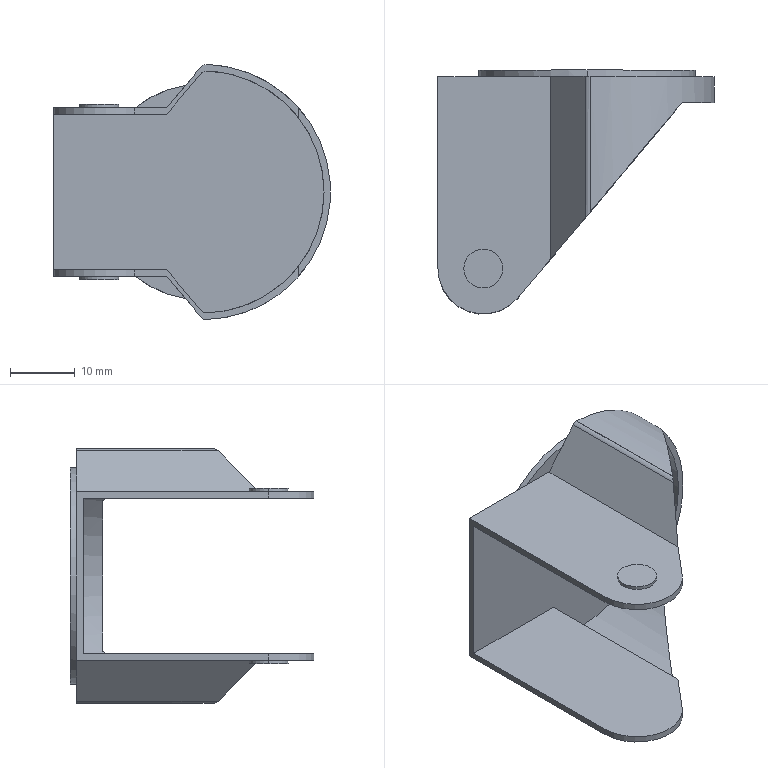Part | STEP file | CLGJ50_Rbody | 1 solid | 36 faces | box 42.667 x 37.625 x 39.322 mm | volume 4018 mm3 | plane 20 | cylinder 16 | commonest cylinder face diameters 2 x6 6 x4 14 x2 33.333 x2 37.333 x1 39.333 x1
STEP:
#1=CARTESIAN_POINT('',(-13.,-40.,-13.5));
#2=VERTEX_POINT('',#1);
#3=CARTESIAN_POINT('',(-19.,-40.,-13.5));
#4=VERTEX_POINT('',#3);
#5=CARTESIAN_POINT('',(-16.,-40.,-13.5));
#6=DIRECTION('',(0.,0.,1.));
#7=DIRECTION('',(1.,0.,0.));
#8=AXIS2_PLACEMENT_3D('',#5,#6,#7);
#9=CIRCLE('',#8,3.);
#10=EDGE_CURVE('',#2,#4,#9,.T.);
#11=ORIENTED_EDGE('',*,*,#10,.T.);
#12=CARTESIAN_POINT('',(-19.,-40.,-13.));
#13=VERTEX_POINT('',#12);
#14=CARTESIAN_POINT('',(-19.,-40.,-13.5));
#15=DIRECTION('',(0.,0.,1.));
#16=VECTOR('',#15,1000.);
#17=LINE('',#14,#16);
#18=EDGE_CURVE('',#4,#13,#17,.T.);
#19=ORIENTED_EDGE('',*,*,#18,.T.);
#20=CARTESIAN_POINT('',(-13.,-40.,-13.));
#21=VERTEX_POINT('',#20);
#22=CARTESIAN_POINT('',(-16.,-40.,-13.));
#23=DIRECTION('',(0.,0.,-1.));
#24=DIRECTION('',(-1.,0.,0.));
#25=AXIS2_PLACEMENT_3D('',#22,#23,#24);
#26=CIRCLE('',#25,3.);
#27=EDGE_CURVE('',#13,#21,#26,.T.);
#28=ORIENTED_EDGE('',*,*,#27,.T.);
#29=CARTESIAN_POINT('',(-13.,-40.,-13.5));
#30=DIRECTION('',(0.,0.,1.));
#31=VECTOR('',#30,1000.);
#32=LINE('',#29,#31);
#33=EDGE_CURVE('',#2,#21,#32,.T.);
#34=ORIENTED_EDGE('',*,*,#33,.F.);
#35=EDGE_LOOP('',(#11,#19,#28,#34));
#36=FACE_OUTER_BOUND('',#35,.T.);
#37=CARTESIAN_POINT('',(-16.,-40.,-13.5));
#38=DIRECTION('',(0.,0.,1.));
#39=DIRECTION('',(1.,0.,0.));
#40=AXIS2_PLACEMENT_3D('',#37,#38,#39);
#41=CYLINDRICAL_SURFACE('',#40,3.);
#42=ADVANCED_FACE('',(#36),#41,.T.);
#43=CARTESIAN_POINT('',(-13.,-40.,13.5));
#44=VERTEX_POINT('',#43);
#45=CARTESIAN_POINT('',(-19.,-40.,13.5));
#46=VERTEX_POINT('',#45);
#47=CARTESIAN_POINT('',(-16.,-40.,13.5));
#48=DIRECTION('',(0.,0.,1.));
#49=DIRECTION('',(1.,0.,0.));
#50=AXIS2_PLACEMENT_3D('',#47,#48,#49);
#51=CIRCLE('',#50,3.);
#52=EDGE_CURVE('',#44,#46,#51,.T.);
#53=ORIENTED_EDGE('',*,*,#52,.F.);
#54=CARTESIAN_POINT('',(-13.,-40.,13.));
#55=VERTEX_POINT('',#54);
#56=CARTESIAN_POINT('',(-13.,-40.,13.5));
#57=DIRECTION('',(0.,0.,-1.));
#58=VECTOR('',#57,1000.);
#59=LINE('',#56,#58);
#60=EDGE_CURVE('',#44,#55,#59,.T.);
#61=ORIENTED_EDGE('',*,*,#60,.T.);
#62=CARTESIAN_POINT('',(-19.,-40.,13.));
#63=VERTEX_POINT('',#62);
#64=CARTESIAN_POINT('',(-16.,-40.,13.));
#65=DIRECTION('',(0.,0.,1.));
#66=DIRECTION('',(1.,0.,0.));
#67=AXIS2_PLACEMENT_3D('',#64,#65,#66);
#68=CIRCLE('',#67,3.);
#69=EDGE_CURVE('',#55,#63,#68,.T.);
#70=ORIENTED_EDGE('',*,*,#69,.T.);
#71=CARTESIAN_POINT('',(-19.,-40.,13.5));
#72=DIRECTION('',(0.,0.,-1.));
#73=VECTOR('',#72,1000.);
#74=LINE('',#71,#73);
#75=EDGE_CURVE('',#46,#63,#74,.T.);
#76=ORIENTED_EDGE('',*,*,#75,.F.);
#77=EDGE_LOOP('',(#53,#61,#70,#76));
#78=FACE_OUTER_BOUND('',#77,.T.);
#79=CARTESIAN_POINT('',(-16.,-40.,13.5));
#80=DIRECTION('',(0.,0.,-1.));
#81=DIRECTION('',(-1.,0.,0.));
#82=AXIS2_PLACEMENT_3D('',#79,#80,#81);
#83=CYLINDRICAL_SURFACE('',#82,3.);
#84=ADVANCED_FACE('',(#78),#83,.T.);
#85=CARTESIAN_POINT('',(0.4874,-31.255,18.66));
#86=VERTEX_POINT('',#85);
#87=CARTESIAN_POINT('',(0.4613,-31.286,18.661));
#88=VERTEX_POINT('',#87);
#89=CARTESIAN_POINT('',(0.4874,-31.255,18.66));
#90=CARTESIAN_POINT('',(0.4787,-31.266,18.661));
#91=CARTESIAN_POINT('',(0.47,-31.276,18.661));
#92=CARTESIAN_POINT('',(0.4613,-31.286,18.661));
#93=(BOUNDED_CURVE()B_SPLINE_CURVE(3,(#89,#90,#91,#92),.UNSPECIFIED.,.F.,.F.)B_SPLINE_CURVE_WITH_KNOTS((4,4),(1.545,1.571),.UNSPECIFIED.)CURVE()GEOMETRIC_REPRESENTATION_ITEM()RATIONAL_B_SPLINE_CURVE((1.,0.9999,0.9999,1.))REPRESENTATION_ITEM(''));
#94=EDGE_CURVE('',#86,#88,#93,.T.);
#95=ORIENTED_EDGE('',*,*,#94,.T.);
#96=CARTESIAN_POINT('',(0.4613,-11.375,18.661));
#97=VERTEX_POINT('',#96);
#98=CARTESIAN_POINT('',(0.4613,-76.375,18.661));
#99=DIRECTION('',(0.,1.,0.));
#100=VECTOR('',#99,1000.);
#101=LINE('',#98,#100);
#102=EDGE_CURVE('',#88,#97,#101,.T.);
#103=ORIENTED_EDGE('',*,*,#102,.T.);
#104=CARTESIAN_POINT('',(0.4874,-11.375,18.66));
#105=VERTEX_POINT('',#104);
#106=CARTESIAN_POINT('',(0.4613,-11.375,17.661));
#107=DIRECTION('',(0.,1.,0.));
#108=DIRECTION('',(0.,0.,1.));
#109=AXIS2_PLACEMENT_3D('',#106,#107,#108);
#110=CIRCLE('',#109,1.);
#111=EDGE_CURVE('',#97,#105,#110,.T.);
#112=ORIENTED_EDGE('',*,*,#111,.T.);
#113=CARTESIAN_POINT('',(0.4874,-76.375,18.66));
#114=DIRECTION('',(0.,1.,0.));
#115=VECTOR('',#114,1000.);
#116=LINE('',#113,#115);
#117=EDGE_CURVE('',#86,#105,#116,.T.);
#118=ORIENTED_EDGE('',*,*,#117,.F.);
#119=EDGE_LOOP('',(#95,#103,#112,#118));
#120=FACE_OUTER_BOUND('',#119,.T.);
#121=CARTESIAN_POINT('',(0.4613,-76.375,17.661));
#122=DIRECTION('',(0.,1.,0.));
#123=DIRECTION('',(0.,0.,1.));
#124=AXIS2_PLACEMENT_3D('',#121,#122,#123);
#125=CYLINDRICAL_SURFACE('',#124,1.);
#126=ADVANCED_FACE('',(#120),#125,.F.);
#127=CARTESIAN_POINT('',(0.4615,-31.286,19.661));
#128=VERTEX_POINT('',#127);
#129=CARTESIAN_POINT('',(-0.3045,-32.198,19.304));
#130=VERTEX_POINT('',#129);
#131=CARTESIAN_POINT('',(0.4615,-31.286,19.661));
#132=CARTESIAN_POINT('',(0.161,-31.644,19.661));
#133=CARTESIAN_POINT('',(-0.1114,-31.968,19.534));
#134=CARTESIAN_POINT('',(-0.3045,-32.198,19.304));
#135=(BOUNDED_CURVE()B_SPLINE_CURVE(3,(#131,#132,#133,#134),.UNSPECIFIED.,.F.,.F.)B_SPLINE_CURVE_WITH_KNOTS((4,4),(1.571,2.443),.UNSPECIFIED.)CURVE()GEOMETRIC_REPRESENTATION_ITEM()RATIONAL_B_SPLINE_CURVE((1.,0.9375,0.9375,1.))REPRESENTATION_ITEM(''));
#136=EDGE_CURVE('',#128,#130,#135,.T.);
#137=ORIENTED_EDGE('',*,*,#136,.F.);
#138=CARTESIAN_POINT('',(0.4615,-10.375,19.661));
#139=VERTEX_POINT('',#138);
#140=CARTESIAN_POINT('',(0.4615,-54.375,19.661));
#141=DIRECTION('',(0.,1.,0.));
#142=VECTOR('',#141,1000.);
#143=LINE('',#140,#142);
#144=EDGE_CURVE('',#128,#139,#143,.T.);
#145=ORIENTED_EDGE('',*,*,#144,.T.);
#146=CARTESIAN_POINT('',(-0.3045,-10.375,19.304));
#147=VERTEX_POINT('',#146);
#148=CARTESIAN_POINT('',(0.4615,-10.375,18.661));
#149=DIRECTION('',(0.,1.,0.));
#150=DIRECTION('',(0.,0.,1.));
#151=AXIS2_PLACEMENT_3D('',#148,#149,#150);
#152=CIRCLE('',#151,1.);
#153=EDGE_CURVE('',#147,#139,#152,.T.);
#154=ORIENTED_EDGE('',*,*,#153,.F.);
#155=CARTESIAN_POINT('',(-0.3045,-54.375,19.304));
#156=DIRECTION('',(0.,1.,0.));
#157=VECTOR('',#156,1000.);
#158=LINE('',#155,#157);
#159=EDGE_CURVE('',#130,#147,#158,.T.);
#160=ORIENTED_EDGE('',*,*,#159,.F.);
#161=EDGE_LOOP('',(#137,#145,#154,#160));
#162=FACE_OUTER_BOUND('',#161,.T.);
#163=CARTESIAN_POINT('',(0.4615,-54.375,18.661));
#164=DIRECTION('',(0.,1.,0.));
#165=DIRECTION('',(0.,0.,1.));
#166=AXIS2_PLACEMENT_3D('',#163,#164,#165);
#167=CYLINDRICAL_SURFACE('',#166,1.);
#168=ADVANCED_FACE('',(#162),#167,.T.);
#169=CARTESIAN_POINT('',(0.,-10.375,16.667));
#170=VERTEX_POINT('',#169);
#171=CARTESIAN_POINT('',(0.,-10.375,-16.667));
#172=VERTEX_POINT('',#171);
#173=CARTESIAN_POINT('',(0.,-10.375,0.));
#174=DIRECTION('',(0.,1.,0.));
#175=DIRECTION('',(0.,0.,1.));
#176=AXIS2_PLACEMENT_3D('',#173,#174,#175);
#177=CIRCLE('',#176,16.667);
#178=EDGE_CURVE('',#170,#172,#177,.T.);
#179=ORIENTED_EDGE('',*,*,#178,.T.);
#180=CARTESIAN_POINT('',(0.,-9.375,-16.667));
#181=VERTEX_POINT('',#180);
#182=CARTESIAN_POINT('',(0.,-10.375,-16.667));
#183=DIRECTION('',(0.,1.,0.));
#184=VECTOR('',#183,1000.);
#185=LINE('',#182,#184);
#186=EDGE_CURVE('',#172,#181,#185,.T.);
#187=ORIENTED_EDGE('',*,*,#186,.T.);
#188=CARTESIAN_POINT('',(0.,-9.375,16.667));
#189=VERTEX_POINT('',#188);
#190=CARTESIAN_POINT('',(0.,-9.375,0.));
#191=DIRECTION('',(0.,1.,0.));
#192=DIRECTION('',(0.,0.,1.));
#193=AXIS2_PLACEMENT_3D('',#190,#191,#192);
#194=CIRCLE('',#193,16.667);
#195=EDGE_CURVE('',#189,#181,#194,.T.);
#196=ORIENTED_EDGE('',*,*,#195,.F.);
#197=CARTESIAN_POINT('',(0.,-10.375,16.667));
#198=DIRECTION('',(0.,1.,0.));
#199=VECTOR('',#198,1000.);
#200=LINE('',#197,#199);
#201=EDGE_CURVE('',#170,#189,#200,.T.);
#202=ORIENTED_EDGE('',*,*,#201,.F.);
#203=EDGE_LOOP('',(#179,#187,#196,#202));
#204=FACE_OUTER_BOUND('',#203,.T.);
#205=CARTESIAN_POINT('',(0.,-10.375,0.));
#206=DIRECTION('',(0.,1.,0.));
#207=DIRECTION('',(0.,0.,1.));
#208=AXIS2_PLACEMENT_3D('',#205,#206,#207);
#209=CYLINDRICAL_SURFACE('',#208,16.667);
#210=ADVANCED_FACE('',(#204),#209,.T.);
#211=CARTESIAN_POINT('',(-10.64,-44.502,13.));
#212=VERTEX_POINT('',#211);
#213=CARTESIAN_POINT('',(-23.,-40.,13.));
#214=VERTEX_POINT('',#213);
#215=CARTESIAN_POINT('',(-16.,-40.,13.));
#216=DIRECTION('',(0.,0.,-1.));
#217=DIRECTION('',(1.,0.,0.));
#218=AXIS2_PLACEMENT_3D('',#215,#216,#217);
#219=CIRCLE('',#218,7.);
#220=EDGE_CURVE('',#212,#214,#219,.T.);
#221=ORIENTED_EDGE('',*,*,#220,.F.);
#222=CARTESIAN_POINT('',(-5.594,-38.495,13.));
#223=VERTEX_POINT('',#222);
#224=CARTESIAN_POINT('',(-20.615,-56.378,13.));
#225=DIRECTION('',(-0.6432,-0.7657,0.));
#226=VECTOR('',#225,1000.);
#227=LINE('',#224,#226);
#228=EDGE_CURVE('',#223,#212,#227,.T.);
#229=ORIENTED_EDGE('',*,*,#228,.F.);
#230=CARTESIAN_POINT('',(-5.594,-10.375,13.));
#231=VERTEX_POINT('',#230);
#232=CARTESIAN_POINT('',(-5.594,-54.375,13.));
#233=DIRECTION('',(0.,1.,0.));
#234=VECTOR('',#233,1000.);
#235=LINE('',#232,#234);
#236=EDGE_CURVE('',#223,#231,#235,.T.);
#237=ORIENTED_EDGE('',*,*,#236,.T.);
#238=CARTESIAN_POINT('',(-10.43,-10.375,13.));
#239=VERTEX_POINT('',#238);
#240=CARTESIAN_POINT('',(-23.,-10.375,13.));
#241=DIRECTION('',(1.,0.,0.));
#242=VECTOR('',#241,1000.);
#243=LINE('',#240,#242);
#244=EDGE_CURVE('',#239,#231,#243,.T.);
#245=ORIENTED_EDGE('',*,*,#244,.F.);
#246=CARTESIAN_POINT('',(-23.,-10.375,13.));
#247=VERTEX_POINT('',#246);
#248=CARTESIAN_POINT('',(-23.,-10.375,13.));
#249=DIRECTION('',(1.,0.,0.));
#250=VECTOR('',#249,1000.);
#251=LINE('',#248,#250);
#252=EDGE_CURVE('',#247,#239,#251,.T.);
#253=ORIENTED_EDGE('',*,*,#252,.F.);
#254=CARTESIAN_POINT('',(-23.,-54.375,13.));
#255=DIRECTION('',(0.,1.,0.));
#256=VECTOR('',#255,1000.);
#257=LINE('',#254,#256);
#258=EDGE_CURVE('',#214,#247,#257,.T.);
#259=ORIENTED_EDGE('',*,*,#258,.F.);
#260=EDGE_LOOP('',(#221,#229,#237,#245,#253,#259));
#261=FACE_OUTER_BOUND('',#260,.T.);
#262=CARTESIAN_POINT('',(-16.,-40.,13.));
#263=DIRECTION('',(0.,0.,1.));
#264=DIRECTION('',(1.,0.,0.));
#265=AXIS2_PLACEMENT_3D('',#262,#263,#264);
#266=CIRCLE('',#265,3.);
#267=EDGE_CURVE('',#63,#55,#266,.T.);
#268=ORIENTED_EDGE('',*,*,#267,.F.);
#269=ORIENTED_EDGE('',*,*,#69,.F.);
#270=EDGE_LOOP('',(#268,#269));
#271=FACE_BOUND('',#270,.T.);
#272=CARTESIAN_POINT('',(-23.,-54.375,13.));
#273=DIRECTION('',(0.,0.,1.));
#274=DIRECTION('',(1.,0.,0.));
#275=AXIS2_PLACEMENT_3D('',#272,#273,#274);
#276=PLANE('',#275);
#277=ADVANCED_FACE('',(#261,#271),#276,.T.);
#278=CARTESIAN_POINT('',(-2.702,-10.375,16.446));
#279=VERTEX_POINT('',#278);
#280=CARTESIAN_POINT('',(0.,-10.375,0.));
#281=DIRECTION('',(0.,1.,0.));
#282=DIRECTION('',(0.,0.,1.));
#283=AXIS2_PLACEMENT_3D('',#280,#281,#282);
#284=CIRCLE('',#283,16.667);
#285=EDGE_CURVE('',#239,#279,#284,.T.);
#286=ORIENTED_EDGE('',*,*,#285,.F.);
#287=ORIENTED_EDGE('',*,*,#244,.T.);
#288=CARTESIAN_POINT('',(-5.594,-10.375,13.));
#289=DIRECTION('',(0.6428,0.,0.766));
#290=VECTOR('',#289,1000.);
#291=LINE('',#288,#290);
#292=EDGE_CURVE('',#231,#279,#291,.T.);
#293=ORIENTED_EDGE('',*,*,#292,.T.);
#294=EDGE_LOOP('',(#286,#287,#293));
#295=FACE_OUTER_BOUND('',#294,.T.);
#296=CARTESIAN_POINT('',(0.,-10.375,0.));
#297=DIRECTION('',(0.,1.,0.));
#298=DIRECTION('',(0.,0.,1.));
#299=AXIS2_PLACEMENT_3D('',#296,#297,#298);
#300=PLANE('',#299);
#301=ADVANCED_FACE('',(#295),#300,.F.);
#302=ORIENTED_EDGE('',*,*,#186,.F.);
#303=CARTESIAN_POINT('',(-2.702,-10.375,-16.446));
#304=VERTEX_POINT('',#303);
#305=CARTESIAN_POINT('',(0.,-10.375,0.));
#306=DIRECTION('',(0.,1.,0.));
#307=DIRECTION('',(0.,0.,1.));
#308=AXIS2_PLACEMENT_3D('',#305,#306,#307);
#309=CIRCLE('',#308,16.667);
#310=EDGE_CURVE('',#172,#304,#309,.T.);
#311=ORIENTED_EDGE('',*,*,#310,.T.);
#312=CARTESIAN_POINT('',(-10.43,-10.375,-13.));
#313=VERTEX_POINT('',#312);
#314=CARTESIAN_POINT('',(0.,-10.375,0.));
#315=DIRECTION('',(0.,1.,0.));
#316=DIRECTION('',(0.,0.,1.));
#317=AXIS2_PLACEMENT_3D('',#314,#315,#316);
#318=CIRCLE('',#317,16.667);
#319=EDGE_CURVE('',#304,#313,#318,.T.);
#320=ORIENTED_EDGE('',*,*,#319,.T.);
#321=CARTESIAN_POINT('',(0.,-10.375,0.));
#322=DIRECTION('',(0.,1.,0.));
#323=DIRECTION('',(0.,0.,1.));
#324=AXIS2_PLACEMENT_3D('',#321,#322,#323);
#325=CIRCLE('',#324,16.667);
#326=EDGE_CURVE('',#313,#239,#325,.T.);
#327=ORIENTED_EDGE('',*,*,#326,.T.);
#328=ORIENTED_EDGE('',*,*,#285,.T.);
#329=CARTESIAN_POINT('',(0.,-10.375,0.));
#330=DIRECTION('',(0.,1.,0.));
#331=DIRECTION('',(0.,0.,1.));
#332=AXIS2_PLACEMENT_3D('',#329,#330,#331);
#333=CIRCLE('',#332,16.667);
#334=EDGE_CURVE('',#279,#170,#333,.T.);
#335=ORIENTED_EDGE('',*,*,#334,.T.);
#336=ORIENTED_EDGE('',*,*,#201,.T.);
#337=CARTESIAN_POINT('',(0.,-9.375,0.));
#338=DIRECTION('',(0.,1.,0.));
#339=DIRECTION('',(0.,0.,1.));
#340=AXIS2_PLACEMENT_3D('',#337,#338,#339);
#341=CIRCLE('',#340,16.667);
#342=EDGE_CURVE('',#181,#189,#341,.T.);
#343=ORIENTED_EDGE('',*,*,#342,.F.);
#344=EDGE_LOOP('',(#302,#311,#320,#327,#328,#335,#336,#343));
#345=FACE_OUTER_BOUND('',#344,.T.);
#346=CARTESIAN_POINT('',(0.,-10.375,0.));
#347=DIRECTION('',(0.,1.,0.));
#348=DIRECTION('',(0.,0.,1.));
#349=AXIS2_PLACEMENT_3D('',#346,#347,#348);
#350=CYLINDRICAL_SURFACE('',#349,16.667);
#351=ADVANCED_FACE('',(#345),#350,.T.);
#352=CARTESIAN_POINT('',(-5.594,-10.375,-13.));
#353=VERTEX_POINT('',#352);
#354=CARTESIAN_POINT('',(-0.3045,-10.375,-19.304));
#355=DIRECTION('',(-0.6428,0.,0.766));
#356=VECTOR('',#355,1000.);
#357=LINE('',#354,#356);
#358=EDGE_CURVE('',#304,#353,#357,.T.);
#359=ORIENTED_EDGE('',*,*,#358,.T.);
#360=CARTESIAN_POINT('',(-5.594,-10.375,-13.));
#361=DIRECTION('',(-1.,0.,0.));
#362=VECTOR('',#361,1000.);
#363=LINE('',#360,#362);
#364=EDGE_CURVE('',#353,#313,#363,.T.);
#365=ORIENTED_EDGE('',*,*,#364,.T.);
#366=ORIENTED_EDGE('',*,*,#319,.F.);
#367=EDGE_LOOP('',(#359,#365,#366));
#368=FACE_OUTER_BOUND('',#367,.T.);
#369=CARTESIAN_POINT('',(0.,-10.375,0.));
#370=DIRECTION('',(0.,1.,0.));
#371=DIRECTION('',(0.,0.,1.));
#372=AXIS2_PLACEMENT_3D('',#369,#370,#371);
#373=PLANE('',#372);
#374=ADVANCED_FACE('',(#368),#373,.F.);
#375=ORIENTED_EDGE('',*,*,#195,.T.);
#376=ORIENTED_EDGE('',*,*,#342,.T.);
#377=EDGE_LOOP('',(#375,#376));
#378=FACE_OUTER_BOUND('',#377,.T.);
#379=CARTESIAN_POINT('',(0.,-9.375,0.));
#380=DIRECTION('',(0.,1.,0.));
#381=DIRECTION('',(0.,0.,1.));
#382=AXIS2_PLACEMENT_3D('',#379,#380,#381);
#383=PLANE('',#382);
#384=ADVANCED_FACE('',(#378),#383,.T.);
#385=ORIENTED_EDGE('',*,*,#326,.F.);
#386=CARTESIAN_POINT('',(-23.,-10.375,-13.));
#387=VERTEX_POINT('',#386);
#388=CARTESIAN_POINT('',(-5.594,-10.375,-13.));
#389=DIRECTION('',(-1.,0.,0.));
#390=VECTOR('',#389,1000.);
#391=LINE('',#388,#390);
#392=EDGE_CURVE('',#313,#387,#391,.T.);
#393=ORIENTED_EDGE('',*,*,#392,.T.);
#394=CARTESIAN_POINT('',(-23.,-10.375,-13.));
#395=DIRECTION('',(0.,0.,1.));
#396=VECTOR('',#395,1000.);
#397=LINE('',#394,#396);
#398=EDGE_CURVE('',#387,#247,#397,.T.);
#399=ORIENTED_EDGE('',*,*,#398,.T.);
#400=ORIENTED_EDGE('',*,*,#252,.T.);
#401=EDGE_LOOP('',(#385,#393,#399,#400));
#402=FACE_OUTER_BOUND('',#401,.T.);
#403=CARTESIAN_POINT('',(0.4615,-10.375,18.661));
#404=DIRECTION('',(0.,1.,0.));
#405=DIRECTION('',(0.,0.,1.));
#406=AXIS2_PLACEMENT_3D('',#403,#404,#405);
#407=PLANE('',#406);
#408=ADVANCED_FACE('',(#402),#407,.T.);
#409=ORIENTED_EDGE('',*,*,#334,.F.);
#410=CARTESIAN_POINT('',(-5.594,-10.375,13.));
#411=DIRECTION('',(0.6428,0.,0.766));
#412=VECTOR('',#411,1000.);
#413=LINE('',#410,#412);
#414=EDGE_CURVE('',#279,#147,#413,.T.);
#415=ORIENTED_EDGE('',*,*,#414,.T.);
#416=ORIENTED_EDGE('',*,*,#153,.T.);
#417=CARTESIAN_POINT('',(0.4862,-10.375,19.661));
#418=VERTEX_POINT('',#417);
#419=CARTESIAN_POINT('',(0.4615,-10.375,18.661));
#420=DIRECTION('',(0.,1.,0.));
#421=DIRECTION('',(0.,0.,1.));
#422=AXIS2_PLACEMENT_3D('',#419,#420,#421);
#423=CIRCLE('',#422,1.);
#424=EDGE_CURVE('',#139,#418,#423,.T.);
#425=ORIENTED_EDGE('',*,*,#424,.T.);
#426=CARTESIAN_POINT('',(0.4862,-10.375,-19.661));
#427=VERTEX_POINT('',#426);
#428=CARTESIAN_POINT('',(0.,-10.375,0.));
#429=DIRECTION('',(0.,1.,0.));
#430=DIRECTION('',(0.,0.,1.));
#431=AXIS2_PLACEMENT_3D('',#428,#429,#430);
#432=CIRCLE('',#431,19.667);
#433=EDGE_CURVE('',#418,#427,#432,.T.);
#434=ORIENTED_EDGE('',*,*,#433,.T.);
#435=CARTESIAN_POINT('',(-0.3045,-10.375,-19.304));
#436=VERTEX_POINT('',#435);
#437=CARTESIAN_POINT('',(0.4615,-10.375,-18.661));
#438=DIRECTION('',(0.,1.,0.));
#439=DIRECTION('',(0.,0.,1.));
#440=AXIS2_PLACEMENT_3D('',#437,#438,#439);
#441=CIRCLE('',#440,1.);
#442=EDGE_CURVE('',#427,#436,#441,.T.);
#443=ORIENTED_EDGE('',*,*,#442,.T.);
#444=CARTESIAN_POINT('',(-0.3045,-10.375,-19.304));
#445=DIRECTION('',(-0.6428,0.,0.766));
#446=VECTOR('',#445,1000.);
#447=LINE('',#444,#446);
#448=EDGE_CURVE('',#436,#304,#447,.T.);
#449=ORIENTED_EDGE('',*,*,#448,.T.);
#450=ORIENTED_EDGE('',*,*,#310,.F.);
#451=ORIENTED_EDGE('',*,*,#178,.F.);
#452=EDGE_LOOP('',(#409,#415,#416,#425,#434,#443,#449,#450,#451));
#453=FACE_OUTER_BOUND('',#452,.T.);
#454=CARTESIAN_POINT('',(0.4615,-10.375,18.661));
#455=DIRECTION('',(0.,1.,0.));
#456=DIRECTION('',(0.,0.,1.));
#457=AXIS2_PLACEMENT_3D('',#454,#455,#456);
#458=PLANE('',#457);
#459=ADVANCED_FACE('',(#453),#458,.T.);
#460=CARTESIAN_POINT('',(-16.,-40.,-13.));
#461=DIRECTION('',(0.,0.,-1.));
#462=DIRECTION('',(-1.,0.,0.));
#463=AXIS2_PLACEMENT_3D('',#460,#461,#462);
#464=CIRCLE('',#463,3.);
#465=EDGE_CURVE('',#21,#13,#464,.T.);
#466=ORIENTED_EDGE('',*,*,#465,.F.);
#467=ORIENTED_EDGE('',*,*,#27,.F.);
#468=EDGE_LOOP('',(#466,#467));
#469=FACE_BOUND('',#468,.T.);
#470=CARTESIAN_POINT('',(-23.,-40.,-13.));
#471=VERTEX_POINT('',#470);
#472=CARTESIAN_POINT('',(-10.64,-44.502,-13.));
#473=VERTEX_POINT('',#472);
#474=CARTESIAN_POINT('',(-16.,-40.,-13.));
#475=DIRECTION('',(0.,0.,1.));
#476=DIRECTION('',(-1.,0.,0.));
#477=AXIS2_PLACEMENT_3D('',#474,#475,#476);
#478=CIRCLE('',#477,7.);
#479=EDGE_CURVE('',#471,#473,#478,.T.);
#480=ORIENTED_EDGE('',*,*,#479,.F.);
#481=CARTESIAN_POINT('',(-23.,-54.375,-13.));
#482=DIRECTION('',(0.,1.,0.));
#483=VECTOR('',#482,1000.);
#484=LINE('',#481,#483);
#485=EDGE_CURVE('',#471,#387,#484,.T.);
#486=ORIENTED_EDGE('',*,*,#485,.T.);
#487=ORIENTED_EDGE('',*,*,#392,.F.);
#488=ORIENTED_EDGE('',*,*,#364,.F.);
#489=CARTESIAN_POINT('',(-5.594,-38.495,-13.));
#490=VERTEX_POINT('',#489);
#491=CARTESIAN_POINT('',(-5.594,-54.375,-13.));
#492=DIRECTION('',(0.,1.,0.));
#493=VECTOR('',#492,1000.);
#494=LINE('',#491,#493);
#495=EDGE_CURVE('',#490,#353,#494,.T.);
#496=ORIENTED_EDGE('',*,*,#495,.F.);
#497=CARTESIAN_POINT('',(-13.415,-47.806,-13.));
#498=DIRECTION('',(0.6432,0.7657,0.));
#499=VECTOR('',#498,1000.);
#500=LINE('',#497,#499);
#501=EDGE_CURVE('',#473,#490,#500,.T.);
#502=ORIENTED_EDGE('',*,*,#501,.F.);
#503=EDGE_LOOP('',(#480,#486,#487,#488,#496,#502));
#504=FACE_OUTER_BOUND('',#503,.T.);
#505=CARTESIAN_POINT('',(-5.594,-54.375,-13.));
#506=DIRECTION('',(0.,0.,-1.));
#507=DIRECTION('',(-1.,0.,0.));
#508=AXIS2_PLACEMENT_3D('',#505,#506,#507);
#509=PLANE('',#508);
#510=ADVANCED_FACE('',(#469,#504),#509,.T.);
#511=CARTESIAN_POINT('',(-0.3045,-32.198,-19.304));
#512=VERTEX_POINT('',#511);
#513=CARTESIAN_POINT('',(-7.184,-40.388,-11.105));
#514=DIRECTION('',(0.5105,0.6077,-0.6084));
#515=VECTOR('',#514,1000.);
#516=LINE('',#513,#515);
#517=EDGE_CURVE('',#490,#512,#516,.T.);
#518=ORIENTED_EDGE('',*,*,#517,.F.);
#519=ORIENTED_EDGE('',*,*,#495,.T.);
#520=ORIENTED_EDGE('',*,*,#358,.F.);
#521=ORIENTED_EDGE('',*,*,#448,.F.);
#522=CARTESIAN_POINT('',(-0.3045,-54.375,-19.304));
#523=DIRECTION('',(0.,1.,0.));
#524=VECTOR('',#523,1000.);
#525=LINE('',#522,#524);
#526=EDGE_CURVE('',#512,#436,#525,.T.);
#527=ORIENTED_EDGE('',*,*,#526,.F.);
#528=EDGE_LOOP('',(#518,#519,#520,#521,#527));
#529=FACE_OUTER_BOUND('',#528,.T.);
#530=CARTESIAN_POINT('',(-0.3045,-54.375,-19.304));
#531=DIRECTION('',(-0.766,0.,-0.6428));
#532=DIRECTION('',(-0.6428,0.,0.766));
#533=AXIS2_PLACEMENT_3D('',#530,#531,#532);
#534=PLANE('',#533);
#535=ADVANCED_FACE('',(#529),#534,.T.);
#536=CARTESIAN_POINT('',(0.4862,-31.257,-19.661));
#537=VERTEX_POINT('',#536);
#538=CARTESIAN_POINT('',(-0.3045,-32.198,-19.304));
#539=CARTESIAN_POINT('',(-0.1055,-31.961,-19.541));
#540=CARTESIAN_POINT('',(0.1767,-31.625,-19.668));
#541=CARTESIAN_POINT('',(0.4862,-31.257,-19.661));
#542=(BOUNDED_CURVE()B_SPLINE_CURVE(3,(#538,#539,#540,#541),.UNSPECIFIED.,.F.,.F.)B_SPLINE_CURVE_WITH_KNOTS((4,4),(3.84,4.737),.UNSPECIFIED.)CURVE()GEOMETRIC_REPRESENTATION_ITEM()RATIONAL_B_SPLINE_CURVE((1.,0.934,0.934,1.))REPRESENTATION_ITEM(''));
#543=EDGE_CURVE('',#512,#537,#542,.T.);
#544=ORIENTED_EDGE('',*,*,#543,.F.);
#545=ORIENTED_EDGE('',*,*,#526,.T.);
#546=ORIENTED_EDGE('',*,*,#442,.F.);
#547=CARTESIAN_POINT('',(0.4862,-54.375,-19.661));
#548=DIRECTION('',(0.,1.,0.));
#549=VECTOR('',#548,1000.);
#550=LINE('',#547,#549);
#551=EDGE_CURVE('',#537,#427,#550,.T.);
#552=ORIENTED_EDGE('',*,*,#551,.F.);
#553=EDGE_LOOP('',(#544,#545,#546,#552));
#554=FACE_OUTER_BOUND('',#553,.T.);
#555=CARTESIAN_POINT('',(0.4615,-54.375,-18.661));
#556=DIRECTION('',(0.,1.,0.));
#557=DIRECTION('',(0.,0.,1.));
#558=AXIS2_PLACEMENT_3D('',#555,#556,#557);
#559=CYLINDRICAL_SURFACE('',#558,1.);
#560=ADVANCED_FACE('',(#554),#559,.T.);
#561=CARTESIAN_POINT('',(14.667,-14.375,13.102));
#562=VERTEX_POINT('',#561);
#563=CARTESIAN_POINT('',(0.4862,-31.257,19.661));
#564=VERTEX_POINT('',#563);
#565=CARTESIAN_POINT('',(14.667,-14.375,13.102));
#566=CARTESIAN_POINT('',(10.996,-18.745,17.211));
#567=CARTESIAN_POINT('',(5.995,-24.699,19.524));
#568=CARTESIAN_POINT('',(0.4862,-31.257,19.661));
#569=(BOUNDED_CURVE()B_SPLINE_CURVE(3,(#565,#566,#567,#568),.UNSPECIFIED.,.F.,.F.)B_SPLINE_CURVE_WITH_KNOTS((4,4),(0.7291,1.546),.UNSPECIFIED.)CURVE()GEOMETRIC_REPRESENTATION_ITEM()RATIONAL_B_SPLINE_CURVE((1.,0.9452,0.9452,1.))REPRESENTATION_ITEM(''));
#570=EDGE_CURVE('',#562,#564,#569,.T.);
#571=ORIENTED_EDGE('',*,*,#570,.F.);
#572=CARTESIAN_POINT('',(14.667,-14.375,-13.102));
#573=VERTEX_POINT('',#572);
#574=CARTESIAN_POINT('',(0.,-14.375,0.));
#575=DIRECTION('',(0.,-1.,0.));
#576=DIRECTION('',(0.,0.,1.));
#577=AXIS2_PLACEMENT_3D('',#574,#575,#576);
#578=CIRCLE('',#577,19.667);
#579=EDGE_CURVE('',#573,#562,#578,.T.);
#580=ORIENTED_EDGE('',*,*,#579,.F.);
#581=CARTESIAN_POINT('',(0.4862,-31.257,-19.661));
#582=CARTESIAN_POINT('',(5.995,-24.699,-19.524));
#583=CARTESIAN_POINT('',(10.996,-18.745,-17.211));
#584=CARTESIAN_POINT('',(14.667,-14.375,-13.102));
#585=(BOUNDED_CURVE()B_SPLINE_CURVE(3,(#581,#582,#583,#584),.UNSPECIFIED.,.F.,.F.)B_SPLINE_CURVE_WITH_KNOTS((4,4),(4.737,5.554),.UNSPECIFIED.)CURVE()GEOMETRIC_REPRESENTATION_ITEM()RATIONAL_B_SPLINE_CURVE((1.,0.9452,0.9452,1.))REPRESENTATION_ITEM(''));
#586=EDGE_CURVE('',#537,#573,#585,.T.);
#587=ORIENTED_EDGE('',*,*,#586,.F.);
#588=ORIENTED_EDGE('',*,*,#551,.T.);
#589=ORIENTED_EDGE('',*,*,#433,.F.);
#590=CARTESIAN_POINT('',(0.4862,-54.375,19.661));
#591=DIRECTION('',(0.,1.,0.));
#592=VECTOR('',#591,1000.);
#593=LINE('',#590,#592);
#594=EDGE_CURVE('',#564,#418,#593,.T.);
#595=ORIENTED_EDGE('',*,*,#594,.F.);
#596=EDGE_LOOP('',(#571,#580,#587,#588,#589,#595));
#597=FACE_OUTER_BOUND('',#596,.T.);
#598=CARTESIAN_POINT('',(0.,-54.375,0.));
#599=DIRECTION('',(0.,1.,0.));
#600=DIRECTION('',(0.,0.,1.));
#601=AXIS2_PLACEMENT_3D('',#598,#599,#600);
#602=CYLINDRICAL_SURFACE('',#601,19.667);
#603=ADVANCED_FACE('',(#597),#602,.T.);
#604=ORIENTED_EDGE('',*,*,#144,.F.);
#605=CARTESIAN_POINT('',(0.4862,-31.257,19.661));
#606=CARTESIAN_POINT('',(0.478,-31.266,19.661));
#607=CARTESIAN_POINT('',(0.4698,-31.276,19.661));
#608=CARTESIAN_POINT('',(0.4615,-31.286,19.661));
#609=(BOUNDED_CURVE()B_SPLINE_CURVE(3,(#605,#606,#607,#608),.UNSPECIFIED.,.F.,.F.)B_SPLINE_CURVE_WITH_KNOTS((4,4),(1.546,1.571),.UNSPECIFIED.)CURVE()GEOMETRIC_REPRESENTATION_ITEM()RATIONAL_B_SPLINE_CURVE((1.,0.9999,0.9999,1.))REPRESENTATION_ITEM(''));
#610=EDGE_CURVE('',#564,#128,#609,.T.);
#611=ORIENTED_EDGE('',*,*,#610,.F.);
#612=ORIENTED_EDGE('',*,*,#594,.T.);
#613=ORIENTED_EDGE('',*,*,#424,.F.);
#614=EDGE_LOOP('',(#604,#611,#612,#613));
#615=FACE_OUTER_BOUND('',#614,.T.);
#616=CARTESIAN_POINT('',(0.4615,-54.375,18.661));
#617=DIRECTION('',(0.,1.,0.));
#618=DIRECTION('',(0.,0.,1.));
#619=AXIS2_PLACEMENT_3D('',#616,#617,#618);
#620=CYLINDRICAL_SURFACE('',#619,1.);
#621=ADVANCED_FACE('',(#615),#620,.T.);
#622=CARTESIAN_POINT('',(-10.52,-44.36,7.129));
#623=DIRECTION('',(-0.5105,-0.6077,-0.6084));
#624=VECTOR('',#623,1000.);
#625=LINE('',#622,#624);
#626=EDGE_CURVE('',#130,#223,#625,.T.);
#627=ORIENTED_EDGE('',*,*,#626,.F.);
#628=ORIENTED_EDGE('',*,*,#159,.T.);
#629=ORIENTED_EDGE('',*,*,#414,.F.);
#630=ORIENTED_EDGE('',*,*,#292,.F.);
#631=ORIENTED_EDGE('',*,*,#236,.F.);
#632=EDGE_LOOP('',(#627,#628,#629,#630,#631));
#633=FACE_OUTER_BOUND('',#632,.T.);
#634=CARTESIAN_POINT('',(-5.594,-54.375,13.));
#635=DIRECTION('',(-0.766,0.,0.6428));
#636=DIRECTION('',(0.6428,0.,0.766));
#637=AXIS2_PLACEMENT_3D('',#634,#635,#636);
#638=PLANE('',#637);
#639=ADVANCED_FACE('',(#633),#638,.T.);
#640=CARTESIAN_POINT('',(-23.,-11.375,-12.));
#641=VERTEX_POINT('',#640);
#642=CARTESIAN_POINT('',(-23.,-11.375,12.));
#643=VERTEX_POINT('',#642);
#644=CARTESIAN_POINT('',(-23.,-11.375,-12.));
#645=DIRECTION('',(0.,0.,1.));
#646=VECTOR('',#645,1000.);
#647=LINE('',#644,#646);
#648=EDGE_CURVE('',#641,#643,#647,.T.);
#649=ORIENTED_EDGE('',*,*,#648,.T.);
#650=CARTESIAN_POINT('',(-23.,-40.,12.));
#651=VERTEX_POINT('',#650);
#652=CARTESIAN_POINT('',(-23.,-76.375,12.));
#653=DIRECTION('',(0.,1.,0.));
#654=VECTOR('',#653,1000.);
#655=LINE('',#652,#654);
#656=EDGE_CURVE('',#651,#643,#655,.T.);
#657=ORIENTED_EDGE('',*,*,#656,.F.);
#658=CARTESIAN_POINT('',(-23.,-40.,-29.5));
#659=DIRECTION('',(0.,0.,1.));
#660=VECTOR('',#659,1000.);
#661=LINE('',#658,#660);
#662=EDGE_CURVE('',#651,#214,#661,.T.);
#663=ORIENTED_EDGE('',*,*,#662,.T.);
#664=ORIENTED_EDGE('',*,*,#258,.T.);
#665=ORIENTED_EDGE('',*,*,#398,.F.);
#666=ORIENTED_EDGE('',*,*,#485,.F.);
#667=CARTESIAN_POINT('',(-23.,-40.,-12.));
#668=VERTEX_POINT('',#667);
#669=CARTESIAN_POINT('',(-23.,-40.,-29.5));
#670=DIRECTION('',(0.,0.,1.));
#671=VECTOR('',#670,1000.);
#672=LINE('',#669,#671);
#673=EDGE_CURVE('',#471,#668,#672,.T.);
#674=ORIENTED_EDGE('',*,*,#673,.T.);
#675=CARTESIAN_POINT('',(-23.,-76.375,-12.));
#676=DIRECTION('',(0.,1.,0.));
#677=VECTOR('',#676,1000.);
#678=LINE('',#675,#677);
#679=EDGE_CURVE('',#668,#641,#678,.T.);
#680=ORIENTED_EDGE('',*,*,#679,.T.);
#681=EDGE_LOOP('',(#649,#657,#663,#664,#665,#666,#674,#680));
#682=FACE_OUTER_BOUND('',#681,.T.);
#683=CARTESIAN_POINT('',(-23.,-54.375,-13.));
#684=DIRECTION('',(-1.,0.,0.));
#685=DIRECTION('',(0.,0.,1.));
#686=AXIS2_PLACEMENT_3D('',#683,#684,#685);
#687=PLANE('',#686);
#688=ADVANCED_FACE('',(#682),#687,.T.);
#689=ORIENTED_EDGE('',*,*,#679,.F.);
#690=CARTESIAN_POINT('',(-10.64,-44.502,-12.));
#691=VERTEX_POINT('',#690);
#692=CARTESIAN_POINT('',(-16.,-40.,-12.));
#693=DIRECTION('',(0.,0.,1.));
#694=DIRECTION('',(-1.,0.,0.));
#695=AXIS2_PLACEMENT_3D('',#692,#693,#694);
#696=CIRCLE('',#695,7.);
#697=EDGE_CURVE('',#668,#691,#696,.T.);
#698=ORIENTED_EDGE('',*,*,#697,.T.);
#699=CARTESIAN_POINT('',(-5.594,-38.495,-12.));
#700=VERTEX_POINT('',#699);
#701=CARTESIAN_POINT('',(-24.25,-60.704,-12.));
#702=DIRECTION('',(0.6432,0.7657,0.));
#703=VECTOR('',#702,1000.);
#704=LINE('',#701,#703);
#705=EDGE_CURVE('',#691,#700,#704,.T.);
#706=ORIENTED_EDGE('',*,*,#705,.T.);
#707=CARTESIAN_POINT('',(-5.594,-11.375,-12.));
#708=VERTEX_POINT('',#707);
#709=CARTESIAN_POINT('',(-5.594,-76.375,-12.));
#710=DIRECTION('',(0.,1.,0.));
#711=VECTOR('',#710,1000.);
#712=LINE('',#709,#711);
#713=EDGE_CURVE('',#700,#708,#712,.T.);
#714=ORIENTED_EDGE('',*,*,#713,.T.);
#715=CARTESIAN_POINT('',(-5.594,-11.375,-12.));
#716=DIRECTION('',(-1.,0.,0.));
#717=VECTOR('',#716,1000.);
#718=LINE('',#715,#717);
#719=EDGE_CURVE('',#708,#641,#718,.T.);
#720=ORIENTED_EDGE('',*,*,#719,.T.);
#721=EDGE_LOOP('',(#689,#698,#706,#714,#720));
#722=FACE_OUTER_BOUND('',#721,.T.);
#723=CARTESIAN_POINT('',(-5.594,-76.375,-12.));
#724=DIRECTION('',(0.,0.,-1.));
#725=DIRECTION('',(-1.,0.,0.));
#726=AXIS2_PLACEMENT_3D('',#723,#724,#725);
#727=PLANE('',#726);
#728=ADVANCED_FACE('',(#722),#727,.F.);
#729=ORIENTED_EDGE('',*,*,#713,.F.);
#730=CARTESIAN_POINT('',(-0.3048,-32.198,-18.303));
#731=VERTEX_POINT('',#730);
#732=CARTESIAN_POINT('',(-14.009,-48.513,-1.971));
#733=DIRECTION('',(0.5105,0.6077,-0.6084));
#734=VECTOR('',#733,1000.);
#735=LINE('',#732,#734);
#736=EDGE_CURVE('',#700,#731,#735,.T.);
#737=ORIENTED_EDGE('',*,*,#736,.T.);
#738=CARTESIAN_POINT('',(-0.3048,-11.375,-18.303));
#739=VERTEX_POINT('',#738);
#740=CARTESIAN_POINT('',(-0.3048,-76.375,-18.303));
#741=DIRECTION('',(0.,1.,0.));
#742=VECTOR('',#741,1000.);
#743=LINE('',#740,#742);
#744=EDGE_CURVE('',#731,#739,#743,.T.);
#745=ORIENTED_EDGE('',*,*,#744,.T.);
#746=CARTESIAN_POINT('',(-0.3048,-11.375,-18.303));
#747=DIRECTION('',(-0.6428,0.,0.766));
#748=VECTOR('',#747,1000.);
#749=LINE('',#746,#748);
#750=EDGE_CURVE('',#739,#708,#749,.T.);
#751=ORIENTED_EDGE('',*,*,#750,.T.);
#752=EDGE_LOOP('',(#729,#737,#745,#751));
#753=FACE_OUTER_BOUND('',#752,.T.);
#754=CARTESIAN_POINT('',(-0.3048,-76.375,-18.303));
#755=DIRECTION('',(-0.766,0.,-0.6428));
#756=DIRECTION('',(-0.6428,0.,0.766));
#757=AXIS2_PLACEMENT_3D('',#754,#755,#756);
#758=PLANE('',#757);
#759=ADVANCED_FACE('',(#753),#758,.F.);
#760=ORIENTED_EDGE('',*,*,#744,.F.);
#761=CARTESIAN_POINT('',(0.4874,-31.255,-18.66));
#762=VERTEX_POINT('',#761);
#763=CARTESIAN_POINT('',(-0.3048,-32.198,-18.303));
#764=CARTESIAN_POINT('',(-0.1054,-31.961,-18.541));
#765=CARTESIAN_POINT('',(0.1773,-31.624,-18.668));
#766=CARTESIAN_POINT('',(0.4874,-31.255,-18.66));
#767=(BOUNDED_CURVE()B_SPLINE_CURVE(3,(#763,#764,#765,#766),.UNSPECIFIED.,.F.,.F.)B_SPLINE_CURVE_WITH_KNOTS((4,4),(3.84,4.739),.UNSPECIFIED.)CURVE()GEOMETRIC_REPRESENTATION_ITEM()RATIONAL_B_SPLINE_CURVE((1.,0.9338,0.9338,1.))REPRESENTATION_ITEM(''));
#768=EDGE_CURVE('',#731,#762,#767,.T.);
#769=ORIENTED_EDGE('',*,*,#768,.T.);
#770=CARTESIAN_POINT('',(0.4874,-11.375,-18.66));
#771=VERTEX_POINT('',#770);
#772=CARTESIAN_POINT('',(0.4874,-76.375,-18.66));
#773=DIRECTION('',(0.,1.,0.));
#774=VECTOR('',#773,1000.);
#775=LINE('',#772,#774);
#776=EDGE_CURVE('',#762,#771,#775,.T.);
#777=ORIENTED_EDGE('',*,*,#776,.T.);
#778=CARTESIAN_POINT('',(0.4613,-11.375,-17.661));
#779=DIRECTION('',(0.,1.,0.));
#780=DIRECTION('',(0.,0.,1.));
#781=AXIS2_PLACEMENT_3D('',#778,#779,#780);
#782=CIRCLE('',#781,1.);
#783=EDGE_CURVE('',#771,#739,#782,.T.);
#784=ORIENTED_EDGE('',*,*,#783,.T.);
#785=EDGE_LOOP('',(#760,#769,#777,#784));
#786=FACE_OUTER_BOUND('',#785,.T.);
#787=CARTESIAN_POINT('',(0.4613,-76.375,-17.661));
#788=DIRECTION('',(0.,1.,0.));
#789=DIRECTION('',(0.,0.,1.));
#790=AXIS2_PLACEMENT_3D('',#787,#788,#789);
#791=CYLINDRICAL_SURFACE('',#790,1.);
#792=ADVANCED_FACE('',(#786),#791,.F.);
#793=CARTESIAN_POINT('',(14.667,-14.375,-11.547));
#794=VERTEX_POINT('',#793);
#795=CARTESIAN_POINT('',(14.667,-14.375,11.547));
#796=VERTEX_POINT('',#795);
#797=CARTESIAN_POINT('',(0.,-14.375,0.));
#798=DIRECTION('',(0.,-1.,0.));
#799=DIRECTION('',(0.,0.,1.));
#800=AXIS2_PLACEMENT_3D('',#797,#798,#799);
#801=CIRCLE('',#800,18.667);
#802=EDGE_CURVE('',#794,#796,#801,.T.);
#803=ORIENTED_EDGE('',*,*,#802,.T.);
#804=CARTESIAN_POINT('',(14.667,-14.375,11.547));
#805=CARTESIAN_POINT('',(11.175,-18.532,15.982));
#806=CARTESIAN_POINT('',(6.13,-24.538,18.513));
#807=CARTESIAN_POINT('',(0.4874,-31.255,18.66));
#808=(BOUNDED_CURVE()B_SPLINE_CURVE(3,(#804,#805,#806,#807),.UNSPECIFIED.,.F.,.F.)B_SPLINE_CURVE_WITH_KNOTS((4,4),(0.6669,1.545),.UNSPECIFIED.)CURVE()GEOMETRIC_REPRESENTATION_ITEM()RATIONAL_B_SPLINE_CURVE((1.,0.9368,0.9368,1.))REPRESENTATION_ITEM(''));
#809=EDGE_CURVE('',#796,#86,#808,.T.);
#810=ORIENTED_EDGE('',*,*,#809,.T.);
#811=ORIENTED_EDGE('',*,*,#117,.T.);
#812=CARTESIAN_POINT('',(0.,-11.375,0.));
#813=DIRECTION('',(0.,1.,0.));
#814=DIRECTION('',(0.,0.,1.));
#815=AXIS2_PLACEMENT_3D('',#812,#813,#814);
#816=CIRCLE('',#815,18.667);
#817=EDGE_CURVE('',#105,#771,#816,.T.);
#818=ORIENTED_EDGE('',*,*,#817,.T.);
#819=ORIENTED_EDGE('',*,*,#776,.F.);
#820=CARTESIAN_POINT('',(0.4874,-31.255,-18.66));
#821=CARTESIAN_POINT('',(6.13,-24.538,-18.513));
#822=CARTESIAN_POINT('',(11.175,-18.532,-15.982));
#823=CARTESIAN_POINT('',(14.667,-14.375,-11.547));
#824=(BOUNDED_CURVE()B_SPLINE_CURVE(3,(#820,#821,#822,#823),.UNSPECIFIED.,.F.,.T.)B_SPLINE_CURVE_WITH_KNOTS((4,4),(4.739,5.616),.UNSPECIFIED.)CURVE()GEOMETRIC_REPRESENTATION_ITEM()RATIONAL_B_SPLINE_CURVE((1.,0.9368,0.9368,1.))REPRESENTATION_ITEM(''));
#825=EDGE_CURVE('',#762,#794,#824,.T.);
#826=ORIENTED_EDGE('',*,*,#825,.T.);
#827=EDGE_LOOP('',(#803,#810,#811,#818,#819,#826));
#828=FACE_OUTER_BOUND('',#827,.T.);
#829=CARTESIAN_POINT('',(0.,-76.375,0.));
#830=DIRECTION('',(0.,1.,0.));
#831=DIRECTION('',(0.,0.,1.));
#832=AXIS2_PLACEMENT_3D('',#829,#830,#831);
#833=CYLINDRICAL_SURFACE('',#832,18.667);
#834=ADVANCED_FACE('',(#828),#833,.F.);
#835=ORIENTED_EDGE('',*,*,#102,.F.);
#836=CARTESIAN_POINT('',(-0.3048,-32.198,18.303));
#837=VERTEX_POINT('',#836);
#838=CARTESIAN_POINT('',(0.4613,-31.286,18.661));
#839=CARTESIAN_POINT('',(0.1607,-31.644,18.661));
#840=CARTESIAN_POINT('',(-0.1116,-31.968,18.534));
#841=CARTESIAN_POINT('',(-0.3048,-32.198,18.303));
#842=(BOUNDED_CURVE()B_SPLINE_CURVE(3,(#838,#839,#840,#841),.UNSPECIFIED.,.F.,.F.)B_SPLINE_CURVE_WITH_KNOTS((4,4),(1.571,2.443),.UNSPECIFIED.)CURVE()GEOMETRIC_REPRESENTATION_ITEM()RATIONAL_B_SPLINE_CURVE((1.,0.9375,0.9375,1.))REPRESENTATION_ITEM(''));
#843=EDGE_CURVE('',#88,#837,#842,.T.);
#844=ORIENTED_EDGE('',*,*,#843,.T.);
#845=CARTESIAN_POINT('',(-0.3048,-11.375,18.303));
#846=VERTEX_POINT('',#845);
#847=CARTESIAN_POINT('',(-0.3048,-76.375,18.303));
#848=DIRECTION('',(0.,1.,0.));
#849=VECTOR('',#848,1000.);
#850=LINE('',#847,#849);
#851=EDGE_CURVE('',#837,#846,#850,.T.);
#852=ORIENTED_EDGE('',*,*,#851,.T.);
#853=CARTESIAN_POINT('',(0.4613,-11.375,17.661));
#854=DIRECTION('',(0.,1.,0.));
#855=DIRECTION('',(0.,0.,1.));
#856=AXIS2_PLACEMENT_3D('',#853,#854,#855);
#857=CIRCLE('',#856,1.);
#858=EDGE_CURVE('',#846,#97,#857,.T.);
#859=ORIENTED_EDGE('',*,*,#858,.T.);
#860=EDGE_LOOP('',(#835,#844,#852,#859));
#861=FACE_OUTER_BOUND('',#860,.T.);
#862=CARTESIAN_POINT('',(0.4613,-76.375,17.661));
#863=DIRECTION('',(0.,1.,0.));
#864=DIRECTION('',(0.,0.,1.));
#865=AXIS2_PLACEMENT_3D('',#862,#863,#864);
#866=CYLINDRICAL_SURFACE('',#865,1.);
#867=ADVANCED_FACE('',(#861),#866,.F.);
#868=ORIENTED_EDGE('',*,*,#851,.F.);
#869=CARTESIAN_POINT('',(-5.594,-38.495,12.));
#870=VERTEX_POINT('',#869);
#871=CARTESIAN_POINT('',(-17.345,-52.485,-2.005));
#872=DIRECTION('',(-0.5105,-0.6077,-0.6084));
#873=VECTOR('',#872,1000.);
#874=LINE('',#871,#873);
#875=EDGE_CURVE('',#837,#870,#874,.T.);
#876=ORIENTED_EDGE('',*,*,#875,.T.);
#877=CARTESIAN_POINT('',(-5.594,-11.375,12.));
#878=VERTEX_POINT('',#877);
#879=CARTESIAN_POINT('',(-5.594,-76.375,12.));
#880=DIRECTION('',(0.,1.,0.));
#881=VECTOR('',#880,1000.);
#882=LINE('',#879,#881);
#883=EDGE_CURVE('',#870,#878,#882,.T.);
#884=ORIENTED_EDGE('',*,*,#883,.T.);
#885=CARTESIAN_POINT('',(-5.594,-11.375,12.));
#886=DIRECTION('',(0.6428,0.,0.766));
#887=VECTOR('',#886,1000.);
#888=LINE('',#885,#887);
#889=EDGE_CURVE('',#878,#846,#888,.T.);
#890=ORIENTED_EDGE('',*,*,#889,.T.);
#891=EDGE_LOOP('',(#868,#876,#884,#890));
#892=FACE_OUTER_BOUND('',#891,.T.);
#893=CARTESIAN_POINT('',(-5.594,-76.375,12.));
#894=DIRECTION('',(-0.766,0.,0.6428));
#895=DIRECTION('',(0.6428,0.,0.766));
#896=AXIS2_PLACEMENT_3D('',#893,#894,#895);
#897=PLANE('',#896);
#898=ADVANCED_FACE('',(#892),#897,.F.);
#899=CARTESIAN_POINT('',(-10.64,-44.502,12.));
#900=VERTEX_POINT('',#899);
#901=CARTESIAN_POINT('',(-31.45,-69.277,12.));
#902=DIRECTION('',(-0.6432,-0.7657,0.));
#903=VECTOR('',#902,1000.);
#904=LINE('',#901,#903);
#905=EDGE_CURVE('',#870,#900,#904,.T.);
#906=ORIENTED_EDGE('',*,*,#905,.T.);
#907=CARTESIAN_POINT('',(-16.,-40.,12.));
#908=DIRECTION('',(0.,0.,-1.));
#909=DIRECTION('',(1.,0.,0.));
#910=AXIS2_PLACEMENT_3D('',#907,#908,#909);
#911=CIRCLE('',#910,7.);
#912=EDGE_CURVE('',#900,#651,#911,.T.);
#913=ORIENTED_EDGE('',*,*,#912,.T.);
#914=ORIENTED_EDGE('',*,*,#656,.T.);
#915=CARTESIAN_POINT('',(-23.,-11.375,12.));
#916=DIRECTION('',(1.,0.,0.));
#917=VECTOR('',#916,1000.);
#918=LINE('',#915,#917);
#919=EDGE_CURVE('',#643,#878,#918,.T.);
#920=ORIENTED_EDGE('',*,*,#919,.T.);
#921=ORIENTED_EDGE('',*,*,#883,.F.);
#922=EDGE_LOOP('',(#906,#913,#914,#920,#921));
#923=FACE_OUTER_BOUND('',#922,.T.);
#924=CARTESIAN_POINT('',(-23.,-76.375,12.));
#925=DIRECTION('',(0.,0.,1.));
#926=DIRECTION('',(1.,0.,0.));
#927=AXIS2_PLACEMENT_3D('',#924,#925,#926);
#928=PLANE('',#927);
#929=ADVANCED_FACE('',(#923),#928,.F.);
#930=ORIENTED_EDGE('',*,*,#719,.F.);
#931=ORIENTED_EDGE('',*,*,#750,.F.);
#932=ORIENTED_EDGE('',*,*,#783,.F.);
#933=ORIENTED_EDGE('',*,*,#817,.F.);
#934=ORIENTED_EDGE('',*,*,#111,.F.);
#935=ORIENTED_EDGE('',*,*,#858,.F.);
#936=ORIENTED_EDGE('',*,*,#889,.F.);
#937=ORIENTED_EDGE('',*,*,#919,.F.);
#938=ORIENTED_EDGE('',*,*,#648,.F.);
#939=EDGE_LOOP('',(#930,#931,#932,#933,#934,#935,#936,#937,#938));
#940=FACE_OUTER_BOUND('',#939,.T.);
#941=CARTESIAN_POINT('',(0.4613,-11.375,17.661));
#942=DIRECTION('',(0.,1.,0.));
#943=DIRECTION('',(0.,0.,1.));
#944=AXIS2_PLACEMENT_3D('',#941,#942,#943);
#945=PLANE('',#944);
#946=ADVANCED_FACE('',(#940),#945,.F.);
#947=ORIENTED_EDGE('',*,*,#579,.T.);
#948=CARTESIAN_POINT('',(14.667,-14.375,-29.5));
#949=DIRECTION('',(0.,0.,1.));
#950=VECTOR('',#949,1000.);
#951=LINE('',#948,#950);
#952=EDGE_CURVE('',#796,#562,#951,.T.);
#953=ORIENTED_EDGE('',*,*,#952,.F.);
#954=ORIENTED_EDGE('',*,*,#802,.F.);
#955=CARTESIAN_POINT('',(14.667,-14.375,-29.5));
#956=DIRECTION('',(0.,0.,1.));
#957=VECTOR('',#956,1000.);
#958=LINE('',#955,#957);
#959=EDGE_CURVE('',#573,#794,#958,.T.);
#960=ORIENTED_EDGE('',*,*,#959,.F.);
#961=EDGE_LOOP('',(#947,#953,#954,#960));
#962=FACE_OUTER_BOUND('',#961,.T.);
#963=CARTESIAN_POINT('',(24.667,-14.375,-29.5));
#964=DIRECTION('',(0.,1.,0.));
#965=DIRECTION('',(0.,0.,1.));
#966=AXIS2_PLACEMENT_3D('',#963,#964,#965);
#967=PLANE('',#966);
#968=ADVANCED_FACE('',(#962),#967,.F.);
#969=ORIENTED_EDGE('',*,*,#479,.T.);
#970=CARTESIAN_POINT('',(-10.64,-44.502,-29.5));
#971=DIRECTION('',(0.,0.,1.));
#972=VECTOR('',#971,1000.);
#973=LINE('',#970,#972);
#974=EDGE_CURVE('',#473,#691,#973,.T.);
#975=ORIENTED_EDGE('',*,*,#974,.T.);
#976=ORIENTED_EDGE('',*,*,#697,.F.);
#977=ORIENTED_EDGE('',*,*,#673,.F.);
#978=EDGE_LOOP('',(#969,#975,#976,#977));
#979=FACE_OUTER_BOUND('',#978,.T.);
#980=CARTESIAN_POINT('',(-16.,-40.,-29.5));
#981=DIRECTION('',(0.,0.,1.));
#982=DIRECTION('',(1.,0.,0.));
#983=AXIS2_PLACEMENT_3D('',#980,#981,#982);
#984=CYLINDRICAL_SURFACE('',#983,7.);
#985=ADVANCED_FACE('',(#979),#984,.T.);
#986=ORIENTED_EDGE('',*,*,#220,.T.);
#987=ORIENTED_EDGE('',*,*,#662,.F.);
#988=ORIENTED_EDGE('',*,*,#912,.F.);
#989=CARTESIAN_POINT('',(-10.64,-44.502,-29.5));
#990=DIRECTION('',(0.,0.,1.));
#991=VECTOR('',#990,1000.);
#992=LINE('',#989,#991);
#993=EDGE_CURVE('',#900,#212,#992,.T.);
#994=ORIENTED_EDGE('',*,*,#993,.T.);
#995=EDGE_LOOP('',(#986,#987,#988,#994));
#996=FACE_OUTER_BOUND('',#995,.T.);
#997=CARTESIAN_POINT('',(-16.,-40.,-29.5));
#998=DIRECTION('',(0.,0.,1.));
#999=DIRECTION('',(1.,0.,0.));
#1000=AXIS2_PLACEMENT_3D('',#997,#998,#999);
#1001=CYLINDRICAL_SURFACE('',#1000,7.);
#1002=ADVANCED_FACE('',(#996),#1001,.T.);
#1003=ORIENTED_EDGE('',*,*,#501,.T.);
#1004=ORIENTED_EDGE('',*,*,#517,.T.);
#1005=ORIENTED_EDGE('',*,*,#543,.T.);
#1006=ORIENTED_EDGE('',*,*,#586,.T.);
#1007=ORIENTED_EDGE('',*,*,#959,.T.);
#1008=ORIENTED_EDGE('',*,*,#825,.F.);
#1009=ORIENTED_EDGE('',*,*,#768,.F.);
#1010=ORIENTED_EDGE('',*,*,#736,.F.);
#1011=ORIENTED_EDGE('',*,*,#705,.F.);
#1012=ORIENTED_EDGE('',*,*,#974,.F.);
#1013=EDGE_LOOP('',(#1003,#1004,#1005,#1006,#1007,#1008,#1009,#1010,#1011,#1012));
#1014=FACE_OUTER_BOUND('',#1013,.T.);
#1015=CARTESIAN_POINT('',(14.667,-14.375,-29.5));
#1016=DIRECTION('',(-0.7657,0.6432,0.));
#1017=DIRECTION('',(-0.6432,-0.7657,0.));
#1018=AXIS2_PLACEMENT_3D('',#1015,#1016,#1017);
#1019=PLANE('',#1018);
#1020=ADVANCED_FACE('',(#1014),#1019,.F.);
#1021=ORIENTED_EDGE('',*,*,#570,.T.);
#1022=ORIENTED_EDGE('',*,*,#610,.T.);
#1023=ORIENTED_EDGE('',*,*,#136,.T.);
#1024=ORIENTED_EDGE('',*,*,#626,.T.);
#1025=ORIENTED_EDGE('',*,*,#228,.T.);
#1026=ORIENTED_EDGE('',*,*,#993,.F.);
#1027=ORIENTED_EDGE('',*,*,#905,.F.);
#1028=ORIENTED_EDGE('',*,*,#875,.F.);
#1029=ORIENTED_EDGE('',*,*,#843,.F.);
#1030=ORIENTED_EDGE('',*,*,#94,.F.);
#1031=ORIENTED_EDGE('',*,*,#809,.F.);
#1032=ORIENTED_EDGE('',*,*,#952,.T.);
#1033=EDGE_LOOP('',(#1021,#1022,#1023,#1024,#1025,#1026,#1027,#1028,#1029,#1030,#1031,#1032));
#1034=FACE_OUTER_BOUND('',#1033,.T.);
#1035=CARTESIAN_POINT('',(14.667,-14.375,-29.5));
#1036=DIRECTION('',(-0.7657,0.6432,0.));
#1037=DIRECTION('',(-0.6432,-0.7657,0.));
#1038=AXIS2_PLACEMENT_3D('',#1035,#1036,#1037);
#1039=PLANE('',#1038);
#1040=ADVANCED_FACE('',(#1034),#1039,.F.);
#1041=ORIENTED_EDGE('',*,*,#60,.F.);
#1042=CARTESIAN_POINT('',(-16.,-40.,13.5));
#1043=DIRECTION('',(0.,0.,1.));
#1044=DIRECTION('',(1.,0.,0.));
#1045=AXIS2_PLACEMENT_3D('',#1042,#1043,#1044);
#1046=CIRCLE('',#1045,3.);
#1047=EDGE_CURVE('',#46,#44,#1046,.T.);
#1048=ORIENTED_EDGE('',*,*,#1047,.F.);
#1049=ORIENTED_EDGE('',*,*,#75,.T.);
#1050=ORIENTED_EDGE('',*,*,#267,.T.);
#1051=EDGE_LOOP('',(#1041,#1048,#1049,#1050));
#1052=FACE_OUTER_BOUND('',#1051,.T.);
#1053=CARTESIAN_POINT('',(-16.,-40.,13.5));
#1054=DIRECTION('',(0.,0.,-1.));
#1055=DIRECTION('',(-1.,0.,0.));
#1056=AXIS2_PLACEMENT_3D('',#1053,#1054,#1055);
#1057=CYLINDRICAL_SURFACE('',#1056,3.);
#1058=ADVANCED_FACE('',(#1052),#1057,.T.);
#1059=ORIENTED_EDGE('',*,*,#1047,.T.);
#1060=ORIENTED_EDGE('',*,*,#52,.T.);
#1061=EDGE_LOOP('',(#1059,#1060));
#1062=FACE_OUTER_BOUND('',#1061,.T.);
#1063=CARTESIAN_POINT('',(-16.,-40.,13.5));
#1064=DIRECTION('',(0.,0.,1.));
#1065=DIRECTION('',(1.,0.,0.));
#1066=AXIS2_PLACEMENT_3D('',#1063,#1064,#1065);
#1067=PLANE('',#1066);
#1068=ADVANCED_FACE('',(#1062),#1067,.T.);
#1069=ORIENTED_EDGE('',*,*,#18,.F.);
#1070=CARTESIAN_POINT('',(-16.,-40.,-13.5));
#1071=DIRECTION('',(0.,0.,1.));
#1072=DIRECTION('',(1.,0.,0.));
#1073=AXIS2_PLACEMENT_3D('',#1070,#1071,#1072);
#1074=CIRCLE('',#1073,3.);
#1075=EDGE_CURVE('',#4,#2,#1074,.T.);
#1076=ORIENTED_EDGE('',*,*,#1075,.T.);
#1077=ORIENTED_EDGE('',*,*,#33,.T.);
#1078=ORIENTED_EDGE('',*,*,#465,.T.);
#1079=EDGE_LOOP('',(#1069,#1076,#1077,#1078));
#1080=FACE_OUTER_BOUND('',#1079,.T.);
#1081=CARTESIAN_POINT('',(-16.,-40.,-13.5));
#1082=DIRECTION('',(0.,0.,1.));
#1083=DIRECTION('',(1.,0.,0.));
#1084=AXIS2_PLACEMENT_3D('',#1081,#1082,#1083);
#1085=CYLINDRICAL_SURFACE('',#1084,3.);
#1086=ADVANCED_FACE('',(#1080),#1085,.T.);
#1087=ORIENTED_EDGE('',*,*,#10,.F.);
#1088=ORIENTED_EDGE('',*,*,#1075,.F.);
#1089=EDGE_LOOP('',(#1087,#1088));
#1090=FACE_OUTER_BOUND('',#1089,.T.);
#1091=CARTESIAN_POINT('',(-16.,-40.,-13.5));
#1092=DIRECTION('',(0.,0.,1.));
#1093=DIRECTION('',(1.,0.,0.));
#1094=AXIS2_PLACEMENT_3D('',#1091,#1092,#1093);
#1095=PLANE('',#1094);
#1096=ADVANCED_FACE('',(#1090),#1095,.F.);
#1097=CLOSED_SHELL('',(#42,#84,#126,#168,#210,#277,#301,#351,#374,#384,#408,#459,#510,#535,#560,#603,#621,#639,#688,#728,#759,#792,#834,#867,#898,#929,#946,#968,#985,#1002,#1020,#1040,#1058,#1068,#1086,#1096));
#1098=MANIFOLD_SOLID_BREP('',#1097);
#1099=CARTESIAN_POINT('',(0.,0.,0.));
#1100=DIRECTION('',(0.,0.,1.));
#1101=DIRECTION('',(1.,0.,0.));
#1102=AXIS2_PLACEMENT_3D('',#1099,#1100,#1101);
#1103=(LENGTH_UNIT()NAMED_UNIT(*)SI_UNIT(.MILLI.,.METRE.));
#1104=UNCERTAINTY_MEASURE_WITH_UNIT(LENGTH_MEASURE(0.00001),#1103,'','');
#1105=(NAMED_UNIT(*)PLANE_ANGLE_UNIT()SI_UNIT($,.RADIAN.));
#1106=(NAMED_UNIT(*)SI_UNIT($,.STERADIAN.)SOLID_ANGLE_UNIT());
#1107=(GEOMETRIC_REPRESENTATION_CONTEXT(3)GLOBAL_UNCERTAINTY_ASSIGNED_CONTEXT((#1104))GLOBAL_UNIT_ASSIGNED_CONTEXT((#1103,#1105,#1106))REPRESENTATION_CONTEXT('',''));
#1108=ADVANCED_BREP_SHAPE_REPRESENTATION('',(#1098,#1102),#1107);